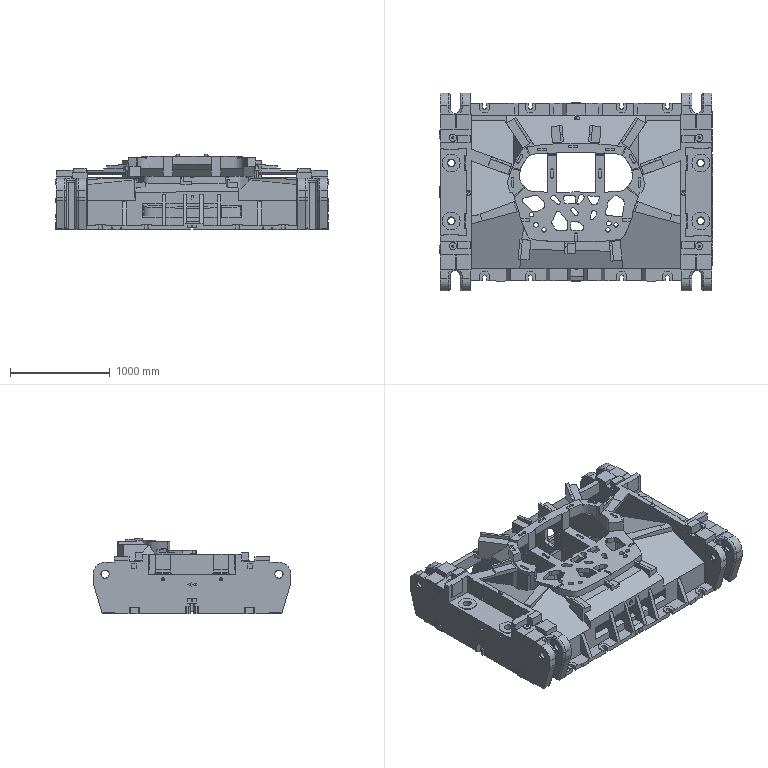Part | NX | features solid 2 | 1 solid | 2265 faces | box 2740 x 1980 x 755 mm | volume 840519292 mm3 | plane 1670 | cylinder 355 | spline 212 | torus 28 | commonest cylinder face diameters 40 x54 60 x52 80 x50 83 x48 25 x27 100 x20